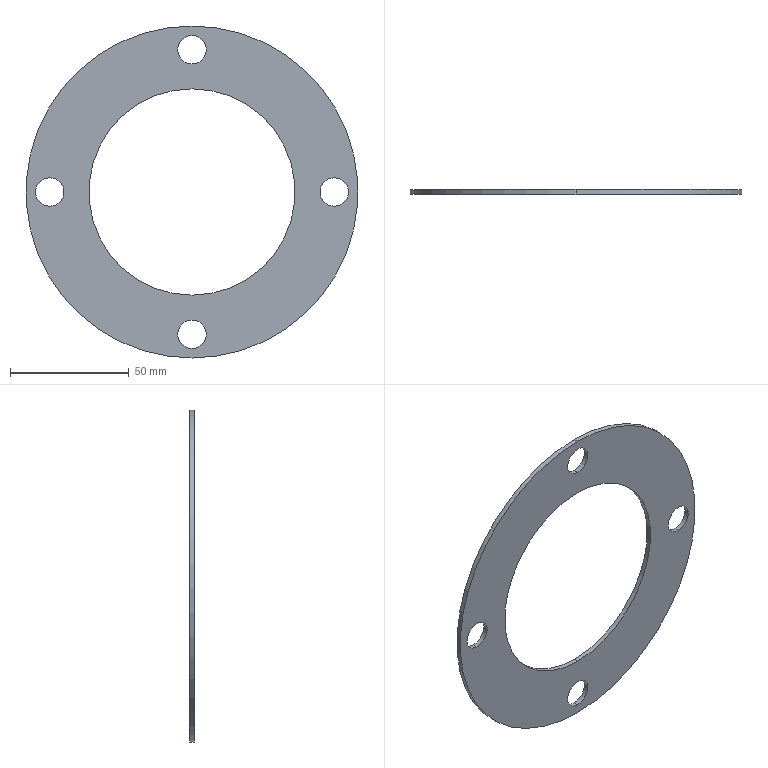Part | SolidWorks | features MirrorStock 1 | 1 solid | 14 faces | box 140 x 2 x 140 mm | volume 17993 mm3 | cylinder 12 | plane 2 | commonest cylinder face diameters 12 x8 87 x2 140 x2
STEP:
#1=CARTESIAN_POINT('',(0.,0.,54.));
#2=VERTEX_POINT('',#1);
#3=CARTESIAN_POINT('',(0.,0.,66.));
#4=VERTEX_POINT('',#3);
#5=CARTESIAN_POINT('',(0.,0.,60.));
#6=DIRECTION('',(0.,-1.,0.));
#7=DIRECTION('',(0.,0.,-1.));
#8=AXIS2_PLACEMENT_3D('',#5,#6,#7);
#9=CIRCLE('',#8,6.);
#10=EDGE_CURVE('',#2,#4,#9,.T.);
#11=ORIENTED_EDGE('',*,*,#10,.T.);
#12=CARTESIAN_POINT('',(0.,2.,66.));
#13=VERTEX_POINT('',#12);
#14=CARTESIAN_POINT('',(0.,0.,66.));
#15=DIRECTION('',(0.,1.,0.));
#16=VECTOR('',#15,1000.);
#17=LINE('',#14,#16);
#18=EDGE_CURVE('',#4,#13,#17,.T.);
#19=ORIENTED_EDGE('',*,*,#18,.T.);
#20=CARTESIAN_POINT('',(0.,2.,54.));
#21=VERTEX_POINT('',#20);
#22=CARTESIAN_POINT('',(0.,2.,60.));
#23=DIRECTION('',(0.,-1.,0.));
#24=DIRECTION('',(0.,0.,-1.));
#25=AXIS2_PLACEMENT_3D('',#22,#23,#24);
#26=CIRCLE('',#25,6.);
#27=EDGE_CURVE('',#21,#13,#26,.T.);
#28=ORIENTED_EDGE('',*,*,#27,.F.);
#29=CARTESIAN_POINT('',(0.,0.,54.));
#30=DIRECTION('',(0.,1.,0.));
#31=VECTOR('',#30,1000.);
#32=LINE('',#29,#31);
#33=EDGE_CURVE('',#2,#21,#32,.T.);
#34=ORIENTED_EDGE('',*,*,#33,.F.);
#35=EDGE_LOOP('',(#11,#19,#28,#34));
#36=FACE_OUTER_BOUND('',#35,.T.);
#37=CARTESIAN_POINT('',(0.,0.,60.));
#38=DIRECTION('',(0.,1.,0.));
#39=DIRECTION('',(0.,0.,-1.));
#40=AXIS2_PLACEMENT_3D('',#37,#38,#39);
#41=CYLINDRICAL_SURFACE('',#40,6.);
#42=ADVANCED_FACE('',(#36),#41,.F.);
#43=CARTESIAN_POINT('',(60.,0.,-6.));
#44=VERTEX_POINT('',#43);
#45=CARTESIAN_POINT('',(60.,0.,6.));
#46=VERTEX_POINT('',#45);
#47=CARTESIAN_POINT('',(60.,0.,0.));
#48=DIRECTION('',(0.,-1.,0.));
#49=DIRECTION('',(0.,0.,-1.));
#50=AXIS2_PLACEMENT_3D('',#47,#48,#49);
#51=CIRCLE('',#50,6.);
#52=EDGE_CURVE('',#44,#46,#51,.T.);
#53=ORIENTED_EDGE('',*,*,#52,.T.);
#54=CARTESIAN_POINT('',(60.,2.,6.));
#55=VERTEX_POINT('',#54);
#56=CARTESIAN_POINT('',(60.,0.,6.));
#57=DIRECTION('',(0.,1.,0.));
#58=VECTOR('',#57,1000.);
#59=LINE('',#56,#58);
#60=EDGE_CURVE('',#46,#55,#59,.T.);
#61=ORIENTED_EDGE('',*,*,#60,.T.);
#62=CARTESIAN_POINT('',(60.,2.,-6.));
#63=VERTEX_POINT('',#62);
#64=CARTESIAN_POINT('',(60.,2.,0.));
#65=DIRECTION('',(0.,-1.,0.));
#66=DIRECTION('',(0.,0.,-1.));
#67=AXIS2_PLACEMENT_3D('',#64,#65,#66);
#68=CIRCLE('',#67,6.);
#69=EDGE_CURVE('',#63,#55,#68,.T.);
#70=ORIENTED_EDGE('',*,*,#69,.F.);
#71=CARTESIAN_POINT('',(60.,0.,-6.));
#72=DIRECTION('',(0.,1.,0.));
#73=VECTOR('',#72,1000.);
#74=LINE('',#71,#73);
#75=EDGE_CURVE('',#44,#63,#74,.T.);
#76=ORIENTED_EDGE('',*,*,#75,.F.);
#77=EDGE_LOOP('',(#53,#61,#70,#76));
#78=FACE_OUTER_BOUND('',#77,.T.);
#79=CARTESIAN_POINT('',(60.,0.,0.));
#80=DIRECTION('',(0.,1.,0.));
#81=DIRECTION('',(0.,0.,-1.));
#82=AXIS2_PLACEMENT_3D('',#79,#80,#81);
#83=CYLINDRICAL_SURFACE('',#82,6.);
#84=ADVANCED_FACE('',(#78),#83,.F.);
#85=CARTESIAN_POINT('',(0.,0.,-66.));
#86=VERTEX_POINT('',#85);
#87=CARTESIAN_POINT('',(0.,0.,-54.));
#88=VERTEX_POINT('',#87);
#89=CARTESIAN_POINT('',(0.,0.,-60.));
#90=DIRECTION('',(0.,-1.,0.));
#91=DIRECTION('',(0.,0.,-1.));
#92=AXIS2_PLACEMENT_3D('',#89,#90,#91);
#93=CIRCLE('',#92,6.);
#94=EDGE_CURVE('',#86,#88,#93,.T.);
#95=ORIENTED_EDGE('',*,*,#94,.T.);
#96=CARTESIAN_POINT('',(0.,2.,-54.));
#97=VERTEX_POINT('',#96);
#98=CARTESIAN_POINT('',(0.,0.,-54.));
#99=DIRECTION('',(0.,1.,0.));
#100=VECTOR('',#99,1000.);
#101=LINE('',#98,#100);
#102=EDGE_CURVE('',#88,#97,#101,.T.);
#103=ORIENTED_EDGE('',*,*,#102,.T.);
#104=CARTESIAN_POINT('',(0.,2.,-66.));
#105=VERTEX_POINT('',#104);
#106=CARTESIAN_POINT('',(0.,2.,-60.));
#107=DIRECTION('',(0.,-1.,0.));
#108=DIRECTION('',(0.,0.,-1.));
#109=AXIS2_PLACEMENT_3D('',#106,#107,#108);
#110=CIRCLE('',#109,6.);
#111=EDGE_CURVE('',#105,#97,#110,.T.);
#112=ORIENTED_EDGE('',*,*,#111,.F.);
#113=CARTESIAN_POINT('',(0.,0.,-66.));
#114=DIRECTION('',(0.,1.,0.));
#115=VECTOR('',#114,1000.);
#116=LINE('',#113,#115);
#117=EDGE_CURVE('',#86,#105,#116,.T.);
#118=ORIENTED_EDGE('',*,*,#117,.F.);
#119=EDGE_LOOP('',(#95,#103,#112,#118));
#120=FACE_OUTER_BOUND('',#119,.T.);
#121=CARTESIAN_POINT('',(0.,0.,-60.));
#122=DIRECTION('',(0.,1.,0.));
#123=DIRECTION('',(0.,0.,-1.));
#124=AXIS2_PLACEMENT_3D('',#121,#122,#123);
#125=CYLINDRICAL_SURFACE('',#124,6.);
#126=ADVANCED_FACE('',(#120),#125,.F.);
#127=CARTESIAN_POINT('',(-60.,0.,-6.));
#128=VERTEX_POINT('',#127);
#129=CARTESIAN_POINT('',(-60.,0.,6.));
#130=VERTEX_POINT('',#129);
#131=CARTESIAN_POINT('',(-60.,0.,0.));
#132=DIRECTION('',(0.,-1.,0.));
#133=DIRECTION('',(0.,0.,-1.));
#134=AXIS2_PLACEMENT_3D('',#131,#132,#133);
#135=CIRCLE('',#134,6.);
#136=EDGE_CURVE('',#128,#130,#135,.T.);
#137=ORIENTED_EDGE('',*,*,#136,.T.);
#138=CARTESIAN_POINT('',(-60.,2.,6.));
#139=VERTEX_POINT('',#138);
#140=CARTESIAN_POINT('',(-60.,0.,6.));
#141=DIRECTION('',(0.,1.,0.));
#142=VECTOR('',#141,1000.);
#143=LINE('',#140,#142);
#144=EDGE_CURVE('',#130,#139,#143,.T.);
#145=ORIENTED_EDGE('',*,*,#144,.T.);
#146=CARTESIAN_POINT('',(-60.,2.,-6.));
#147=VERTEX_POINT('',#146);
#148=CARTESIAN_POINT('',(-60.,2.,0.));
#149=DIRECTION('',(0.,-1.,0.));
#150=DIRECTION('',(0.,0.,-1.));
#151=AXIS2_PLACEMENT_3D('',#148,#149,#150);
#152=CIRCLE('',#151,6.);
#153=EDGE_CURVE('',#147,#139,#152,.T.);
#154=ORIENTED_EDGE('',*,*,#153,.F.);
#155=CARTESIAN_POINT('',(-60.,0.,-6.));
#156=DIRECTION('',(0.,1.,0.));
#157=VECTOR('',#156,1000.);
#158=LINE('',#155,#157);
#159=EDGE_CURVE('',#128,#147,#158,.T.);
#160=ORIENTED_EDGE('',*,*,#159,.F.);
#161=EDGE_LOOP('',(#137,#145,#154,#160));
#162=FACE_OUTER_BOUND('',#161,.T.);
#163=CARTESIAN_POINT('',(-60.,0.,0.));
#164=DIRECTION('',(0.,1.,0.));
#165=DIRECTION('',(0.,0.,-1.));
#166=AXIS2_PLACEMENT_3D('',#163,#164,#165);
#167=CYLINDRICAL_SURFACE('',#166,6.);
#168=ADVANCED_FACE('',(#162),#167,.F.);
#169=CARTESIAN_POINT('',(0.,2.,-43.5));
#170=VERTEX_POINT('',#169);
#171=CARTESIAN_POINT('',(0.,2.,43.5));
#172=VERTEX_POINT('',#171);
#173=CARTESIAN_POINT('',(0.,2.,0.));
#174=DIRECTION('',(0.,-1.,0.));
#175=DIRECTION('',(0.,0.,-1.));
#176=AXIS2_PLACEMENT_3D('',#173,#174,#175);
#177=CIRCLE('',#176,43.5);
#178=EDGE_CURVE('',#170,#172,#177,.T.);
#179=ORIENTED_EDGE('',*,*,#178,.F.);
#180=CARTESIAN_POINT('',(0.,0.,-43.5));
#181=VERTEX_POINT('',#180);
#182=CARTESIAN_POINT('',(0.,2.,-43.5));
#183=DIRECTION('',(0.,-1.,0.));
#184=VECTOR('',#183,1000.);
#185=LINE('',#182,#184);
#186=EDGE_CURVE('',#170,#181,#185,.T.);
#187=ORIENTED_EDGE('',*,*,#186,.T.);
#188=CARTESIAN_POINT('',(0.,0.,43.5));
#189=VERTEX_POINT('',#188);
#190=CARTESIAN_POINT('',(0.,0.,0.));
#191=DIRECTION('',(0.,-1.,0.));
#192=DIRECTION('',(0.,0.,-1.));
#193=AXIS2_PLACEMENT_3D('',#190,#191,#192);
#194=CIRCLE('',#193,43.5);
#195=EDGE_CURVE('',#181,#189,#194,.T.);
#196=ORIENTED_EDGE('',*,*,#195,.T.);
#197=CARTESIAN_POINT('',(0.,2.,43.5));
#198=DIRECTION('',(0.,-1.,0.));
#199=VECTOR('',#198,1000.);
#200=LINE('',#197,#199);
#201=EDGE_CURVE('',#172,#189,#200,.T.);
#202=ORIENTED_EDGE('',*,*,#201,.F.);
#203=EDGE_LOOP('',(#179,#187,#196,#202));
#204=FACE_OUTER_BOUND('',#203,.T.);
#205=CARTESIAN_POINT('',(0.,2.,0.));
#206=DIRECTION('',(0.,-1.,0.));
#207=DIRECTION('',(0.,0.,1.));
#208=AXIS2_PLACEMENT_3D('',#205,#206,#207);
#209=CYLINDRICAL_SURFACE('',#208,43.5);
#210=ADVANCED_FACE('',(#204),#209,.F.);
#211=CARTESIAN_POINT('',(0.,2.,70.));
#212=VERTEX_POINT('',#211);
#213=CARTESIAN_POINT('',(0.,2.,-70.));
#214=VERTEX_POINT('',#213);
#215=CARTESIAN_POINT('',(0.,2.,0.));
#216=DIRECTION('',(0.,-1.,0.));
#217=DIRECTION('',(0.,0.,-1.));
#218=AXIS2_PLACEMENT_3D('',#215,#216,#217);
#219=CIRCLE('',#218,70.);
#220=EDGE_CURVE('',#212,#214,#219,.T.);
#221=ORIENTED_EDGE('',*,*,#220,.T.);
#222=CARTESIAN_POINT('',(0.,0.,-70.));
#223=VERTEX_POINT('',#222);
#224=CARTESIAN_POINT('',(0.,2.,-70.));
#225=DIRECTION('',(0.,-1.,0.));
#226=VECTOR('',#225,1000.);
#227=LINE('',#224,#226);
#228=EDGE_CURVE('',#214,#223,#227,.T.);
#229=ORIENTED_EDGE('',*,*,#228,.T.);
#230=CARTESIAN_POINT('',(0.,0.,70.));
#231=VERTEX_POINT('',#230);
#232=CARTESIAN_POINT('',(0.,0.,0.));
#233=DIRECTION('',(0.,-1.,0.));
#234=DIRECTION('',(0.,0.,-1.));
#235=AXIS2_PLACEMENT_3D('',#232,#233,#234);
#236=CIRCLE('',#235,70.);
#237=EDGE_CURVE('',#231,#223,#236,.T.);
#238=ORIENTED_EDGE('',*,*,#237,.F.);
#239=CARTESIAN_POINT('',(0.,2.,70.));
#240=DIRECTION('',(0.,-1.,0.));
#241=VECTOR('',#240,1000.);
#242=LINE('',#239,#241);
#243=EDGE_CURVE('',#212,#231,#242,.T.);
#244=ORIENTED_EDGE('',*,*,#243,.F.);
#245=EDGE_LOOP('',(#221,#229,#238,#244));
#246=FACE_OUTER_BOUND('',#245,.T.);
#247=CARTESIAN_POINT('',(0.,2.,0.));
#248=DIRECTION('',(0.,-1.,0.));
#249=DIRECTION('',(0.,0.,1.));
#250=AXIS2_PLACEMENT_3D('',#247,#248,#249);
#251=CYLINDRICAL_SURFACE('',#250,70.);
#252=ADVANCED_FACE('',(#246),#251,.T.);
#253=ORIENTED_EDGE('',*,*,#27,.T.);
#254=CARTESIAN_POINT('',(0.,2.,60.));
#255=DIRECTION('',(0.,-1.,0.));
#256=DIRECTION('',(0.,0.,-1.));
#257=AXIS2_PLACEMENT_3D('',#254,#255,#256);
#258=CIRCLE('',#257,6.);
#259=EDGE_CURVE('',#13,#21,#258,.T.);
#260=ORIENTED_EDGE('',*,*,#259,.T.);
#261=EDGE_LOOP('',(#253,#260));
#262=FACE_BOUND('',#261,.T.);
#263=ORIENTED_EDGE('',*,*,#69,.T.);
#264=CARTESIAN_POINT('',(60.,2.,0.));
#265=DIRECTION('',(0.,-1.,0.));
#266=DIRECTION('',(0.,0.,-1.));
#267=AXIS2_PLACEMENT_3D('',#264,#265,#266);
#268=CIRCLE('',#267,6.);
#269=EDGE_CURVE('',#55,#63,#268,.T.);
#270=ORIENTED_EDGE('',*,*,#269,.T.);
#271=EDGE_LOOP('',(#263,#270));
#272=FACE_BOUND('',#271,.T.);
#273=ORIENTED_EDGE('',*,*,#111,.T.);
#274=CARTESIAN_POINT('',(0.,2.,-60.));
#275=DIRECTION('',(0.,-1.,0.));
#276=DIRECTION('',(0.,0.,-1.));
#277=AXIS2_PLACEMENT_3D('',#274,#275,#276);
#278=CIRCLE('',#277,6.);
#279=EDGE_CURVE('',#97,#105,#278,.T.);
#280=ORIENTED_EDGE('',*,*,#279,.T.);
#281=EDGE_LOOP('',(#273,#280));
#282=FACE_BOUND('',#281,.T.);
#283=ORIENTED_EDGE('',*,*,#153,.T.);
#284=CARTESIAN_POINT('',(-60.,2.,0.));
#285=DIRECTION('',(0.,-1.,0.));
#286=DIRECTION('',(0.,0.,-1.));
#287=AXIS2_PLACEMENT_3D('',#284,#285,#286);
#288=CIRCLE('',#287,6.);
#289=EDGE_CURVE('',#139,#147,#288,.T.);
#290=ORIENTED_EDGE('',*,*,#289,.T.);
#291=EDGE_LOOP('',(#283,#290));
#292=FACE_BOUND('',#291,.T.);
#293=ORIENTED_EDGE('',*,*,#220,.F.);
#294=CARTESIAN_POINT('',(0.,2.,0.));
#295=DIRECTION('',(0.,-1.,0.));
#296=DIRECTION('',(0.,0.,-1.));
#297=AXIS2_PLACEMENT_3D('',#294,#295,#296);
#298=CIRCLE('',#297,70.);
#299=EDGE_CURVE('',#214,#212,#298,.T.);
#300=ORIENTED_EDGE('',*,*,#299,.F.);
#301=EDGE_LOOP('',(#293,#300));
#302=FACE_OUTER_BOUND('',#301,.T.);
#303=CARTESIAN_POINT('',(0.,2.,0.));
#304=DIRECTION('',(0.,-1.,0.));
#305=DIRECTION('',(0.,0.,-1.));
#306=AXIS2_PLACEMENT_3D('',#303,#304,#305);
#307=CIRCLE('',#306,43.5);
#308=EDGE_CURVE('',#172,#170,#307,.T.);
#309=ORIENTED_EDGE('',*,*,#308,.T.);
#310=ORIENTED_EDGE('',*,*,#178,.T.);
#311=EDGE_LOOP('',(#309,#310));
#312=FACE_BOUND('',#311,.T.);
#313=CARTESIAN_POINT('',(0.,2.,0.));
#314=DIRECTION('',(0.,1.,0.));
#315=DIRECTION('',(0.,0.,-1.));
#316=AXIS2_PLACEMENT_3D('',#313,#314,#315);
#317=PLANE('',#316);
#318=ADVANCED_FACE('',(#262,#272,#282,#292,#302,#312),#317,.T.);
#319=ORIENTED_EDGE('',*,*,#10,.F.);
#320=CARTESIAN_POINT('',(0.,0.,60.));
#321=DIRECTION('',(0.,-1.,0.));
#322=DIRECTION('',(0.,0.,-1.));
#323=AXIS2_PLACEMENT_3D('',#320,#321,#322);
#324=CIRCLE('',#323,6.);
#325=EDGE_CURVE('',#4,#2,#324,.T.);
#326=ORIENTED_EDGE('',*,*,#325,.F.);
#327=EDGE_LOOP('',(#319,#326));
#328=FACE_BOUND('',#327,.T.);
#329=ORIENTED_EDGE('',*,*,#52,.F.);
#330=CARTESIAN_POINT('',(60.,0.,0.));
#331=DIRECTION('',(0.,-1.,0.));
#332=DIRECTION('',(0.,0.,-1.));
#333=AXIS2_PLACEMENT_3D('',#330,#331,#332);
#334=CIRCLE('',#333,6.);
#335=EDGE_CURVE('',#46,#44,#334,.T.);
#336=ORIENTED_EDGE('',*,*,#335,.F.);
#337=EDGE_LOOP('',(#329,#336));
#338=FACE_BOUND('',#337,.T.);
#339=ORIENTED_EDGE('',*,*,#94,.F.);
#340=CARTESIAN_POINT('',(0.,0.,-60.));
#341=DIRECTION('',(0.,-1.,0.));
#342=DIRECTION('',(0.,0.,-1.));
#343=AXIS2_PLACEMENT_3D('',#340,#341,#342);
#344=CIRCLE('',#343,6.);
#345=EDGE_CURVE('',#88,#86,#344,.T.);
#346=ORIENTED_EDGE('',*,*,#345,.F.);
#347=EDGE_LOOP('',(#339,#346));
#348=FACE_BOUND('',#347,.T.);
#349=ORIENTED_EDGE('',*,*,#136,.F.);
#350=CARTESIAN_POINT('',(-60.,0.,0.));
#351=DIRECTION('',(0.,-1.,0.));
#352=DIRECTION('',(0.,0.,-1.));
#353=AXIS2_PLACEMENT_3D('',#350,#351,#352);
#354=CIRCLE('',#353,6.);
#355=EDGE_CURVE('',#130,#128,#354,.T.);
#356=ORIENTED_EDGE('',*,*,#355,.F.);
#357=EDGE_LOOP('',(#349,#356));
#358=FACE_BOUND('',#357,.T.);
#359=ORIENTED_EDGE('',*,*,#237,.T.);
#360=CARTESIAN_POINT('',(0.,0.,0.));
#361=DIRECTION('',(0.,-1.,0.));
#362=DIRECTION('',(0.,0.,-1.));
#363=AXIS2_PLACEMENT_3D('',#360,#361,#362);
#364=CIRCLE('',#363,70.);
#365=EDGE_CURVE('',#223,#231,#364,.T.);
#366=ORIENTED_EDGE('',*,*,#365,.T.);
#367=EDGE_LOOP('',(#359,#366));
#368=FACE_OUTER_BOUND('',#367,.T.);
#369=CARTESIAN_POINT('',(0.,0.,0.));
#370=DIRECTION('',(0.,-1.,0.));
#371=DIRECTION('',(0.,0.,-1.));
#372=AXIS2_PLACEMENT_3D('',#369,#370,#371);
#373=CIRCLE('',#372,43.5);
#374=EDGE_CURVE('',#189,#181,#373,.T.);
#375=ORIENTED_EDGE('',*,*,#374,.F.);
#376=ORIENTED_EDGE('',*,*,#195,.F.);
#377=EDGE_LOOP('',(#375,#376));
#378=FACE_BOUND('',#377,.T.);
#379=CARTESIAN_POINT('',(0.,0.,0.));
#380=DIRECTION('',(0.,1.,0.));
#381=DIRECTION('',(0.,0.,-1.));
#382=AXIS2_PLACEMENT_3D('',#379,#380,#381);
#383=PLANE('',#382);
#384=ADVANCED_FACE('',(#328,#338,#348,#358,#368,#378),#383,.F.);
#385=ORIENTED_EDGE('',*,*,#228,.F.);
#386=ORIENTED_EDGE('',*,*,#299,.T.);
#387=ORIENTED_EDGE('',*,*,#243,.T.);
#388=ORIENTED_EDGE('',*,*,#365,.F.);
#389=EDGE_LOOP('',(#385,#386,#387,#388));
#390=FACE_OUTER_BOUND('',#389,.T.);
#391=CARTESIAN_POINT('',(0.,2.,0.));
#392=DIRECTION('',(0.,-1.,0.));
#393=DIRECTION('',(0.,0.,1.));
#394=AXIS2_PLACEMENT_3D('',#391,#392,#393);
#395=CYLINDRICAL_SURFACE('',#394,70.);
#396=ADVANCED_FACE('',(#390),#395,.T.);
#397=ORIENTED_EDGE('',*,*,#186,.F.);
#398=ORIENTED_EDGE('',*,*,#308,.F.);
#399=ORIENTED_EDGE('',*,*,#201,.T.);
#400=ORIENTED_EDGE('',*,*,#374,.T.);
#401=EDGE_LOOP('',(#397,#398,#399,#400));
#402=FACE_OUTER_BOUND('',#401,.T.);
#403=CARTESIAN_POINT('',(0.,2.,0.));
#404=DIRECTION('',(0.,-1.,0.));
#405=DIRECTION('',(0.,0.,1.));
#406=AXIS2_PLACEMENT_3D('',#403,#404,#405);
#407=CYLINDRICAL_SURFACE('',#406,43.5);
#408=ADVANCED_FACE('',(#402),#407,.F.);
#409=ORIENTED_EDGE('',*,*,#144,.F.);
#410=ORIENTED_EDGE('',*,*,#355,.T.);
#411=ORIENTED_EDGE('',*,*,#159,.T.);
#412=ORIENTED_EDGE('',*,*,#289,.F.);
#413=EDGE_LOOP('',(#409,#410,#411,#412));
#414=FACE_OUTER_BOUND('',#413,.T.);
#415=CARTESIAN_POINT('',(-60.,0.,0.));
#416=DIRECTION('',(0.,1.,0.));
#417=DIRECTION('',(0.,0.,-1.));
#418=AXIS2_PLACEMENT_3D('',#415,#416,#417);
#419=CYLINDRICAL_SURFACE('',#418,6.);
#420=ADVANCED_FACE('',(#414),#419,.F.);
#421=ORIENTED_EDGE('',*,*,#102,.F.);
#422=ORIENTED_EDGE('',*,*,#345,.T.);
#423=ORIENTED_EDGE('',*,*,#117,.T.);
#424=ORIENTED_EDGE('',*,*,#279,.F.);
#425=EDGE_LOOP('',(#421,#422,#423,#424));
#426=FACE_OUTER_BOUND('',#425,.T.);
#427=CARTESIAN_POINT('',(0.,0.,-60.));
#428=DIRECTION('',(0.,1.,0.));
#429=DIRECTION('',(0.,0.,-1.));
#430=AXIS2_PLACEMENT_3D('',#427,#428,#429);
#431=CYLINDRICAL_SURFACE('',#430,6.);
#432=ADVANCED_FACE('',(#426),#431,.F.);
#433=ORIENTED_EDGE('',*,*,#60,.F.);
#434=ORIENTED_EDGE('',*,*,#335,.T.);
#435=ORIENTED_EDGE('',*,*,#75,.T.);
#436=ORIENTED_EDGE('',*,*,#269,.F.);
#437=EDGE_LOOP('',(#433,#434,#435,#436));
#438=FACE_OUTER_BOUND('',#437,.T.);
#439=CARTESIAN_POINT('',(60.,0.,0.));
#440=DIRECTION('',(0.,1.,0.));
#441=DIRECTION('',(0.,0.,-1.));
#442=AXIS2_PLACEMENT_3D('',#439,#440,#441);
#443=CYLINDRICAL_SURFACE('',#442,6.);
#444=ADVANCED_FACE('',(#438),#443,.F.);
#445=ORIENTED_EDGE('',*,*,#18,.F.);
#446=ORIENTED_EDGE('',*,*,#325,.T.);
#447=ORIENTED_EDGE('',*,*,#33,.T.);
#448=ORIENTED_EDGE('',*,*,#259,.F.);
#449=EDGE_LOOP('',(#445,#446,#447,#448));
#450=FACE_OUTER_BOUND('',#449,.T.);
#451=CARTESIAN_POINT('',(0.,0.,60.));
#452=DIRECTION('',(0.,1.,0.));
#453=DIRECTION('',(0.,0.,-1.));
#454=AXIS2_PLACEMENT_3D('',#451,#452,#453);
#455=CYLINDRICAL_SURFACE('',#454,6.);
#456=ADVANCED_FACE('',(#450),#455,.F.);
#457=CLOSED_SHELL('',(#42,#84,#126,#168,#210,#252,#318,#384,#396,#408,#420,#432,#444,#456));
#458=MANIFOLD_SOLID_BREP('',#457);
#459=CARTESIAN_POINT('',(0.,0.,0.));
#460=DIRECTION('',(0.,0.,1.));
#461=DIRECTION('',(1.,0.,0.));
#462=AXIS2_PLACEMENT_3D('',#459,#460,#461);
#463=(LENGTH_UNIT()NAMED_UNIT(*)SI_UNIT(.MILLI.,.METRE.));
#464=UNCERTAINTY_MEASURE_WITH_UNIT(LENGTH_MEASURE(0.00001),#463,'','');
#465=(NAMED_UNIT(*)PLANE_ANGLE_UNIT()SI_UNIT($,.RADIAN.));
#466=(NAMED_UNIT(*)SI_UNIT($,.STERADIAN.)SOLID_ANGLE_UNIT());
#467=(GEOMETRIC_REPRESENTATION_CONTEXT(3)GLOBAL_UNCERTAINTY_ASSIGNED_CONTEXT((#464))GLOBAL_UNIT_ASSIGNED_CONTEXT((#463,#465,#466))REPRESENTATION_CONTEXT('',''));
#468=ADVANCED_BREP_SHAPE_REPRESENTATION('',(#458,#462),#467);